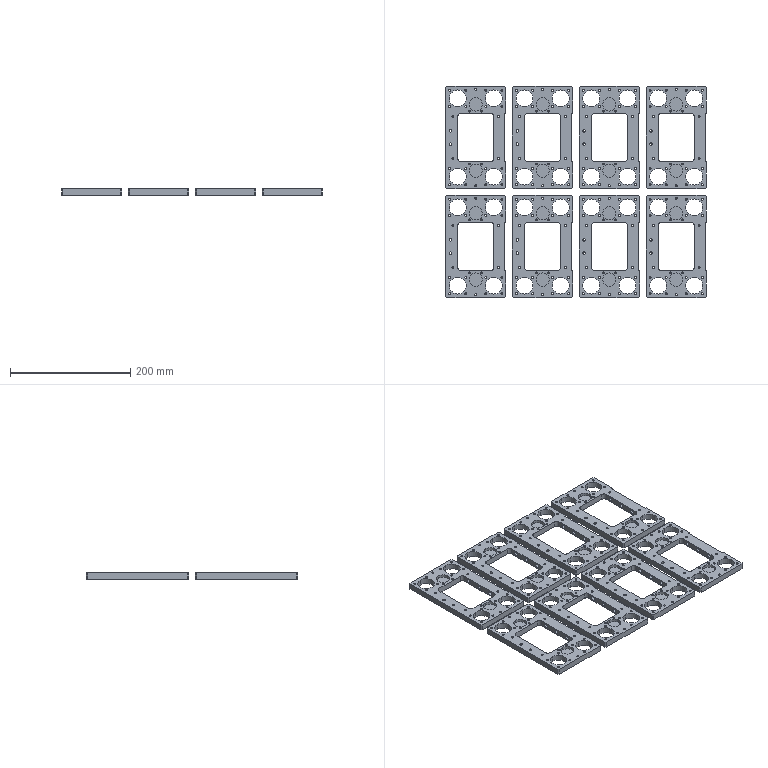NC program | NX | posted with a generic post | part box 433 x 351 x 10 mm
Lines 8361 to 9115 of 15742:
(ZLEVEL_PROFILE_COPY_COPY , TOOL : D10JING)
N16696 T14 M6
N16698 G54
N16700 G17 G0 G90 X191.064 Y-125.4 B0. C0. S9500 M3
N16702 G43 Z30. H14
N16704 Z-8.85
N16706 G94 G1 Z-9.85 F1000.
N16708 G3 X191.5 Y-125.5 R1.
N16710 G1 Y-55.5 F1500.
N16712 X141.623
N16714 X141.5
N16716 Y-125.5
N16718 X191.5
N16720 G3 X191.4 Y-125.064 R1.
N16722 G1 Z-8.85
N16724 G0 Z53.
N16726 X80.064 Y-125.4
N16728 Z-8.85
N16730 G1 Z-9.85 F1000.
N16732 G3 X80.5 Y-125.5 R1.
N16734 G1 Y-55.5 F1500.
N16736 X30.623
N16738 X30.5
N16740 Y-125.5
N16742 X80.5
N16744 G3 X80.4 Y-125.064 R1.
N16746 G1 Z-8.85
N16748 G0 Z53.
N16750 X-30.936 Y-125.4
N16752 Z-8.85
N16754 G1 Z-9.85 F1000.
N16756 G3 X-30.5 Y-125.5 R1.
N16758 G1 Y-55.5 F1500.
N16760 X-30.623
N16762 X-80.377
N16764 X-80.5
N16766 Y-125.5
N16768 X-30.5
N16770 G3 X-30.6 Y-125.064 R1.
N16772 G1 Z-8.85
N16774 G0 Z53.
N16776 X-191.065 Y-55.6
N16778 Z-8.85
N16780 G1 Z-9.85 F1000.
N16782 G3 X-191.5 Y-55.5 R1.
N16784 G1 Y-125.5 F1500.
N16786 X-141.5
N16788 Y-55.5
N16790 X-141.623
N16792 X-191.377
N16794 X-191.5
N16796 G3 X-191.4 Y-55.936 R1.
N16798 G1 Z-8.85
N16800 G0 Z53.
N16802 X-191.065 Y125.4
N16804 Z-8.85
N16806 G1 Z-9.85 F1000.
N16808 G3 X-191.5 Y125.5 R1.
N16810 G1 Y55.5 F1500.
N16812 X-141.5
N16814 Y125.5
N16816 X-141.623
N16818 X-191.377
N16820 X-191.5
N16822 G3 X-191.4 Y125.064 R1.
N16824 G1 Z-8.85
N16826 G0 Z53.
N16828 X-80.065 Y125.4
N16830 Z-8.85
N16832 G1 Z-9.85 F1000.
N16834 G3 X-80.5 Y125.5 R1.
N16836 G1 Y55.5 F1500.
N16838 X-30.5
N16840 Y125.5
N16842 X-30.623
N16844 X-80.377
N16846 X-80.5
N16848 G3 X-80.4 Y125.064 R1.
N16850 G1 Z-8.85
N16852 G0 Z53.
N16854 X30.935 Y125.4
N16856 Z-8.85
N16858 G1 Z-9.85 F1000.
N16860 G3 X30.5 Y125.5 R1.
N16862 G1 Y55.5 F1500.
N16864 X80.5
N16866 Y125.5
N16868 X80.377
N16870 X30.623
N16872 X30.5
N16874 G3 X30.6 Y125.064 R1.
N16876 G1 Z-8.85
N16878 G0 Z53.
N16880 X191.064 Y55.6
N16882 Z-8.85
N16884 G1 Z-9.85 F1000.
N16886 G3 X191.5 Y55.5 R1.
N16888 G1 Y125.5 F1500.
N16890 X191.377
N16892 X141.623
N16894 X141.5
N16896 Y55.5
N16898 X191.5
N16900 G3 X191.4 Y55.936 R1.
N16902 G1 Z-8.85
N16904 G0 Z30.
(HOLE_MILLING , TOOL : D10JING)
N16906 X-196.5 Y-155.5
N16908 Z0.5
N16910 G3 X-194.238 Y-157.763 R2.263 F2200.
N16912 X-191.975 Y-155.5 R2.263
N16914 X-191.975 Y-155.5 Z-0.38 I-4.525 J0.
N16916 X-191.975 Y-155.5 Z-1.26 I-4.525 J0.
N16918 X-191.975 Y-155.5 Z-2.14 I-4.525 J0.
N16920 X-191.975 Y-155.5 Z-3.02 I-4.525 J0.
N16922 X-191.975 Y-155.5 Z-3.9 I-4.525 J0.
N16924 X-191.975 Y-155.5 Z-4.78 I-4.525 J0.
N16926 X-191.975 Y-155.5 Z-5.66 I-4.525 J0.
N16928 X-191.975 Y-155.5 Z-6.54 I-4.525 J0.
N16930 X-191.975 Y-155.5 Z-7.42 I-4.525 J0.
N16932 X-191.975 Y-155.5 Z-8.3 I-4.525 J0.
N16934 X-191.975 Y-155.5 Z-9.18 I-4.525 J0.
N16936 X-192.384 Y-157.38 Z-10. R-4.525
N16938 X-194.62 Y-151.384 R4.525
N16940 X-192.384 Y-157.38 R-4.525
N16942 X-193.502 Y-154.382 R2.263
N16944 X-196.5 Y-155.5 R2.263
N16946 G0 Z0.5
N16948 G3 X-191.975 Y-160.025 R4.525
N16950 X-187.45 Y-155.5 R4.525
N16952 X-187.45 Y-155.5 Z-0.38 I-9.05 J0.
N16954 X-187.45 Y-155.5 Z-1.26 I-9.05 J0.
N16956 X-187.45 Y-155.5 Z-2.14 I-9.05 J0.
N16958 X-187.45 Y-155.5 Z-3.02 I-9.05 J0.
N16960 X-187.45 Y-155.5 Z-3.9 I-9.05 J0.
N16962 X-187.45 Y-155.5 Z-4.78 I-9.05 J0.
N16964 X-187.45 Y-155.5 Z-5.66 I-9.05 J0.
N16966 X-187.45 Y-155.5 Z-6.54 I-9.05 J0.
N16968 X-187.45 Y-155.5 Z-7.42 I-9.05 J0.
N16970 X-187.45 Y-155.5 Z-8.3 I-9.05 J0.
N16972 X-187.45 Y-155.5 Z-9.18 I-9.05 J0.
N16974 X-188.268 Y-159.26 Z-10. R-9.05
N16976 X-192.74 Y-147.268 R9.05
N16978 X-188.268 Y-159.26 R-9.05
N16980 X-190.504 Y-153.264 R4.525
N16982 X-196.5 Y-155.5 R4.525
N16984 G0 Z30.
N16986 X-166.5 Y-145.5
N16988 Z0.5
N16990 G3 X-165. Y-147. R1.5
N16992 X-163.5 Y-145.5 R1.5
N16994 X-163.5 Y-145.5 Z-0.38 I-3. J0.
N16996 X-163.5 Y-145.5 Z-1.26 I-3. J0.
N16998 X-163.5 Y-145.5 Z-2.14 I-3. J0.
N17000 X-163.5 Y-145.5 Z-3.02 I-3. J0.
N17002 X-163.5 Y-145.5 Z-3.9 I-3. J0.
N17004 X-163.5 Y-145.5 Z-4.78 I-3. J0.
N17006 X-166.5 Y-142.5 Z-5. R3.
N17008 X-169.5 Y-145.5 R3.
N17010 X-166.5 Y-142.5 R-3.
N17012 X-168. Y-144. R1.5
N17014 X-166.5 Y-145.5 R1.5
N17016 G0 Z0.5
N17018 G3 X-163.5 Y-148.5 R3.
N17020 X-160.5 Y-145.5 R3.
N17022 X-160.5 Y-145.5 Z-0.38 I-6. J0.
N17024 X-160.5 Y-145.5 Z-1.26 I-6. J0.
N17026 X-160.5 Y-145.5 Z-2.14 I-6. J0.
N17028 X-160.5 Y-145.5 Z-3.02 I-6. J0.
N17030 X-160.5 Y-145.5 Z-3.9 I-6. J0.
N17032 X-160.5 Y-145.5 Z-4.78 I-6. J0.
N17034 X-166.5 Y-139.5 Z-5. R6.
N17036 X-172.5 Y-145.5 R6.
N17038 X-166.5 Y-139.5 R-6.
N17040 X-169.5 Y-142.5 R3.
N17042 X-166.5 Y-145.5 R3.
N17044 G0 Z30.
N17046 X-136.5 Y-155.5
N17048 Z0.5
N17050 G3 X-134.238 Y-157.763 R2.262
N17052 X-131.975 Y-155.5 R2.262
N17054 X-131.975 Y-155.5 Z-0.38 I-4.525 J0.
N17056 X-131.975 Y-155.5 Z-1.26 I-4.525 J0.
N17058 X-131.975 Y-155.5 Z-2.14 I-4.525 J0.
N17060 X-131.975 Y-155.5 Z-3.02 I-4.525 J0.
N17062 X-131.975 Y-155.5 Z-3.9 I-4.525 J0.
N17064 X-131.975 Y-155.5 Z-4.78 I-4.525 J0.
N17066 X-131.975 Y-155.5 Z-5.66 I-4.525 J0.
N17068 X-131.975 Y-155.5 Z-6.54 I-4.525 J0.
N17070 X-131.975 Y-155.5 Z-7.42 I-4.525 J0.
N17072 X-131.975 Y-155.5 Z-8.3 I-4.525 J0.
N17074 X-131.975 Y-155.5 Z-9.18 I-4.525 J0.
N17076 X-132.384 Y-157.38 Z-10. R-4.525
N17078 X-134.62 Y-151.384 R4.525
N17080 X-132.384 Y-157.38 R-4.525
N17082 X-133.502 Y-154.382 R2.263
N17084 X-136.5 Y-155.5 R2.263
N17086 G0 Z0.5
N17088 G3 X-131.975 Y-160.025 R4.525
N17090 X-127.45 Y-155.5 R4.525
N17092 X-127.45 Y-155.5 Z-0.38 I-9.05 J0.
N17094 X-127.45 Y-155.5 Z-1.26 I-9.05 J0.
N17096 X-127.45 Y-155.5 Z-2.14 I-9.05 J0.
N17098 X-127.45 Y-155.5 Z-3.02 I-9.05 J0.
N17100 X-127.45 Y-155.5 Z-3.9 I-9.05 J0.
N17102 X-127.45 Y-155.5 Z-4.78 I-9.05 J0.
N17104 X-127.45 Y-155.5 Z-5.66 I-9.05 J0.
N17106 X-127.45 Y-155.5 Z-6.54 I-9.05 J0.
N17108 X-127.45 Y-155.5 Z-7.42 I-9.05 J0.
N17110 X-127.45 Y-155.5 Z-8.3 I-9.05 J0.
N17112 X-127.45 Y-155.5 Z-9.18 I-9.05 J0.
N17114 X-128.268 Y-159.26 Z-10. R-9.05
N17116 X-132.74 Y-147.268 R9.05
N17118 X-128.268 Y-159.26 R-9.05
N17120 X-130.504 Y-153.264 R4.525
N17122 X-136.5 Y-155.5 R4.525
N17124 G0 Z30.
N17126 X-85.5
N17128 Z0.5
N17130 G3 X-83.238 Y-157.763 R2.263
N17132 X-80.975 Y-155.5 R2.263
N17134 X-80.975 Y-155.5 Z-0.38 I-4.525 J0.
N17136 X-80.975 Y-155.5 Z-1.26 I-4.525 J0.
N17138 X-80.975 Y-155.5 Z-2.14 I-4.525 J0.
N17140 X-80.975 Y-155.5 Z-3.02 I-4.525 J0.
N17142 X-80.975 Y-155.5 Z-3.9 I-4.525 J0.
N17144 X-80.975 Y-155.5 Z-4.78 I-4.525 J0.
N17146 X-80.975 Y-155.5 Z-5.66 I-4.525 J0.
N17148 X-80.975 Y-155.5 Z-6.54 I-4.525 J0.
N17150 X-80.975 Y-155.5 Z-7.42 I-4.525 J0.
N17152 X-80.975 Y-155.5 Z-8.3 I-4.525 J0.
N17154 X-80.975 Y-155.5 Z-9.18 I-4.525 J0.
N17156 X-81.384 Y-157.38 Z-10. R-4.525
N17158 X-83.62 Y-151.384 R4.525
N17160 X-81.384 Y-157.38 R-4.525
N17162 X-82.502 Y-154.382 R2.263
N17164 X-85.5 Y-155.5 R2.263
N17166 G0 Z0.5
N17168 G3 X-80.975 Y-160.025 R4.525
N17170 X-76.45 Y-155.5 R4.525
N17172 X-76.45 Y-155.5 Z-0.38 I-9.05 J0.
N17174 X-76.45 Y-155.5 Z-1.26 I-9.05 J0.
N17176 X-76.45 Y-155.5 Z-2.14 I-9.05 J0.
N17178 X-76.45 Y-155.5 Z-3.02 I-9.05 J0.
N17180 X-76.45 Y-155.5 Z-3.9 I-9.05 J0.
N17182 X-76.45 Y-155.5 Z-4.78 I-9.05 J0.
N17184 X-76.45 Y-155.5 Z-5.66 I-9.05 J0.
N17186 X-76.45 Y-155.5 Z-6.54 I-9.05 J0.
N17188 X-76.45 Y-155.5 Z-7.42 I-9.05 J0.
N17190 X-76.45 Y-155.5 Z-8.3 I-9.05 J0.
N17192 X-76.45 Y-155.5 Z-9.18 I-9.05 J0.
N17194 X-77.268 Y-159.26 Z-10. R-9.05
N17196 X-81.74 Y-147.268 R9.05
N17198 X-77.268 Y-159.26 R-9.05
N17200 X-79.504 Y-153.264 R4.525
N17202 X-85.5 Y-155.5 R4.525
N17204 G0 Z30.
N17206 X-55.5 Y-145.5
N17208 Z0.5
N17210 G3 X-54. Y-147. R1.5
N17212 X-52.5 Y-145.5 R1.5
N17214 X-52.5 Y-145.5 Z-0.38 I-3. J0.
N17216 X-52.5 Y-145.5 Z-1.26 I-3. J0.
N17218 X-52.5 Y-145.5 Z-2.14 I-3. J0.
N17220 X-52.5 Y-145.5 Z-3.02 I-3. J0.
N17222 X-52.5 Y-145.5 Z-3.9 I-3. J0.
N17224 X-52.5 Y-145.5 Z-4.78 I-3. J0.
N17226 X-55.5 Y-142.5 Z-5. R3.
N17228 X-58.5 Y-145.5 R3.
N17230 X-55.5 Y-142.5 R-3.
N17232 X-57. Y-144. R1.5
N17234 X-55.5 Y-145.5 R1.5
N17236 G0 Z0.5
N17238 G3 X-52.5 Y-148.5 R3.
N17240 X-49.5 Y-145.5 R3.
N17242 X-49.5 Y-145.5 Z-0.38 I-6. J0.
N17244 X-49.5 Y-145.5 Z-1.26 I-6. J0.
N17246 X-49.5 Y-145.5 Z-2.14 I-6. J0.
N17248 X-49.5 Y-145.5 Z-3.02 I-6. J0.
N17250 X-49.5 Y-145.5 Z-3.9 I-6. J0.
N17252 X-49.5 Y-145.5 Z-4.78 I-6. J0.
N17254 X-55.5 Y-139.5 Z-5. R6.
N17256 X-61.5 Y-145.5 R6.
N17258 X-55.5 Y-139.5 R-6.
N17260 X-58.5 Y-142.5 R3.
N17262 X-55.5 Y-145.5 R3.
N17264 G0 Z30.
N17266 X-25.5 Y-155.5
N17268 Z0.5
N17270 G3 X-23.238 Y-157.763 R2.263
N17272 X-20.975 Y-155.5 R2.263
N17274 X-20.975 Y-155.5 Z-0.38 I-4.525 J0.
N17276 X-20.975 Y-155.5 Z-1.26 I-4.525 J0.
N17278 X-20.975 Y-155.5 Z-2.14 I-4.525 J0.
N17280 X-20.975 Y-155.5 Z-3.02 I-4.525 J0.
N17282 X-20.975 Y-155.5 Z-3.9 I-4.525 J0.
N17284 X-20.975 Y-155.5 Z-4.78 I-4.525 J0.
N17286 X-20.975 Y-155.5 Z-5.66 I-4.525 J0.
N17288 X-20.975 Y-155.5 Z-6.54 I-4.525 J0.
N17290 X-20.975 Y-155.5 Z-7.42 I-4.525 J0.
N17292 X-20.975 Y-155.5 Z-8.3 I-4.525 J0.
N17294 X-20.975 Y-155.5 Z-9.18 I-4.525 J0.
N17296 X-21.384 Y-157.38 Z-10. R-4.525
N17298 X-23.62 Y-151.384 R4.525
N17300 X-21.384 Y-157.38 R-4.525
N17302 X-22.502 Y-154.382 R2.263
N17304 X-25.5 Y-155.5 R2.263
N17306 G0 Z0.5
N17308 G3 X-20.975 Y-160.025 R4.525
N17310 X-16.45 Y-155.5 R4.525
N17312 X-16.45 Y-155.5 Z-0.38 I-9.05 J0.
N17314 X-16.45 Y-155.5 Z-1.26 I-9.05 J0.
N17316 X-16.45 Y-155.5 Z-2.14 I-9.05 J0.
N17318 X-16.45 Y-155.5 Z-3.02 I-9.05 J0.
N17320 X-16.45 Y-155.5 Z-3.9 I-9.05 J0.
N17322 X-16.45 Y-155.5 Z-4.78 I-9.05 J0.
N17324 X-16.45 Y-155.5 Z-5.66 I-9.05 J0.
N17326 X-16.45 Y-155.5 Z-6.54 I-9.05 J0.
N17328 X-16.45 Y-155.5 Z-7.42 I-9.05 J0.
N17330 X-16.45 Y-155.5 Z-8.3 I-9.05 J0.
N17332 X-16.45 Y-155.5 Z-9.18 I-9.05 J0.
N17334 X-17.268 Y-159.26 Z-10. R-9.05
N17336 X-21.74 Y-147.268 R9.05
N17338 X-17.268 Y-159.26 R-9.05
N17340 X-19.504 Y-153.264 R4.525
N17342 X-25.5 Y-155.5 R4.525
N17344 G0 Z30.
N17346 X25.5
N17348 Z0.5
N17350 G3 X27.763 Y-157.763 R2.263
N17352 X30.025 Y-155.5 R2.263
N17354 X30.025 Y-155.5 Z-0.38 I-4.525 J0.
N17356 X30.025 Y-155.5 Z-1.26 I-4.525 J0.
N17358 X30.025 Y-155.5 Z-2.14 I-4.525 J0.
N17360 X30.025 Y-155.5 Z-3.02 I-4.525 J0.
N17362 X30.025 Y-155.5 Z-3.9 I-4.525 J0.
N17364 X30.025 Y-155.5 Z-4.78 I-4.525 J0.
N17366 X30.025 Y-155.5 Z-5.66 I-4.525 J0.
N17368 X30.025 Y-155.5 Z-6.54 I-4.525 J0.
N17370 X30.025 Y-155.5 Z-7.42 I-4.525 J0.
N17372 X30.025 Y-155.5 Z-8.3 I-4.525 J0.
N17374 X30.025 Y-155.5 Z-9.18 I-4.525 J0.
N17376 X29.616 Y-157.38 Z-10. R-4.525
N17378 X27.38 Y-151.384 R4.525
N17380 X29.616 Y-157.38 R-4.525
N17382 X28.498 Y-154.382 R2.263
N17384 X25.5 Y-155.5 R2.263
N17386 G0 Z0.5
N17388 G3 X30.025 Y-160.025 R4.525
N17390 X34.55 Y-155.5 R4.525
N17392 X34.55 Y-155.5 Z-0.38 I-9.05 J0.
N17394 X34.55 Y-155.5 Z-1.26 I-9.05 J0.
N17396 X34.55 Y-155.5 Z-2.14 I-9.05 J0.
N17398 X34.55 Y-155.5 Z-3.02 I-9.05 J0.
N17400 X34.55 Y-155.5 Z-3.9 I-9.05 J0.
N17402 X34.55 Y-155.5 Z-4.78 I-9.05 J0.
N17404 X34.55 Y-155.5 Z-5.66 I-9.05 J0.
N17406 X34.55 Y-155.5 Z-6.54 I-9.05 J0.
N17408 X34.55 Y-155.5 Z-7.42 I-9.05 J0.
N17410 X34.55 Y-155.5 Z-8.3 I-9.05 J0.
N17412 X34.55 Y-155.5 Z-9.18 I-9.05 J0.
N17414 X33.732 Y-159.26 Z-10. R-9.05
N17416 X29.26 Y-147.268 R9.05
N17418 X33.732 Y-159.26 R-9.05
N17420 X31.496 Y-153.264 R4.525
N17422 X25.5 Y-155.5 R4.525
N17424 G0 Z30.
N17426 X55.5 Y-145.5
N17428 Z0.5
N17430 G3 X57. Y-147. R1.5
N17432 X58.5 Y-145.5 R1.5
N17434 X58.5 Y-145.5 Z-0.38 I-3. J0.
N17436 X58.5 Y-145.5 Z-1.26 I-3. J0.
N17438 X58.5 Y-145.5 Z-2.14 I-3. J0.
N17440 X58.5 Y-145.5 Z-3.02 I-3. J0.
N17442 X58.5 Y-145.5 Z-3.9 I-3. J0.
N17444 X58.5 Y-145.5 Z-4.78 I-3. J0.
N17446 X55.5 Y-142.5 Z-5. R3.
N17448 X52.5 Y-145.5 R3.
N17450 X55.5 Y-142.5 R-3.
N17452 X54. Y-144. R1.5
N17454 X55.5 Y-145.5 R1.5
N17456 G0 Z0.5
N17458 G3 X58.5 Y-148.5 R3.
N17460 X61.5 Y-145.5 R3.
N17462 X61.5 Y-145.5 Z-0.38 I-6. J0.
N17464 X61.5 Y-145.5 Z-1.26 I-6. J0.
N17466 X61.5 Y-145.5 Z-2.14 I-6. J0.
N17468 X61.5 Y-145.5 Z-3.02 I-6. J0.
N17470 X61.5 Y-145.5 Z-3.9 I-6. J0.
N17472 X61.5 Y-145.5 Z-4.78 I-6. J0.
N17474 X55.5 Y-139.5 Z-5. R6.
N17476 X49.5 Y-145.5 R6.
N17478 X55.5 Y-139.5 R-6.
N17480 X52.5 Y-142.5 R3.
N17482 X55.5 Y-145.5 R3.
N17484 G0 Z30.
N17486 X85.5 Y-155.5
N17488 Z0.5
N17490 G3 X87.763 Y-157.763 R2.262
N17492 X90.025 Y-155.5 R2.262
N17494 X90.025 Y-155.5 Z-0.38 I-4.525 J0.
N17496 X90.025 Y-155.5 Z-1.26 I-4.525 J0.
N17498 X90.025 Y-155.5 Z-2.14 I-4.525 J0.
N17500 X90.025 Y-155.5 Z-3.02 I-4.525 J0.
N17502 X90.025 Y-155.5 Z-3.9 I-4.525 J0.
N17504 X90.025 Y-155.5 Z-4.78 I-4.525 J0.
N17506 X90.025 Y-155.5 Z-5.66 I-4.525 J0.
N17508 X90.025 Y-155.5 Z-6.54 I-4.525 J0.
N17510 X90.025 Y-155.5 Z-7.42 I-4.525 J0.
N17512 X90.025 Y-155.5 Z-8.3 I-4.525 J0.
N17514 X90.025 Y-155.5 Z-9.18 I-4.525 J0.
N17516 X89.616 Y-157.38 Z-10. R-4.525
N17518 X87.38 Y-151.384 R4.525
N17520 X89.616 Y-157.38 R-4.525
N17522 X88.498 Y-154.382 R2.263
N17524 X85.5 Y-155.5 R2.263
N17526 G0 Z0.5
N17528 G3 X90.025 Y-160.025 R4.525
N17530 X94.55 Y-155.5 R4.525
N17532 X94.55 Y-155.5 Z-0.38 I-9.05 J0.
N17534 X94.55 Y-155.5 Z-1.26 I-9.05 J0.
N17536 X94.55 Y-155.5 Z-2.14 I-9.05 J0.
N17538 X94.55 Y-155.5 Z-3.02 I-9.05 J0.
N17540 X94.55 Y-155.5 Z-3.9 I-9.05 J0.
N17542 X94.55 Y-155.5 Z-4.78 I-9.05 J0.
N17544 X94.55 Y-155.5 Z-5.66 I-9.05 J0.
N17546 X94.55 Y-155.5 Z-6.54 I-9.05 J0.
N17548 X94.55 Y-155.5 Z-7.42 I-9.05 J0.
N17550 X94.55 Y-155.5 Z-8.3 I-9.05 J0.
N17552 X94.55 Y-155.5 Z-9.18 I-9.05 J0.
N17554 X93.732 Y-159.26 Z-10. R-9.05
N17556 X89.26 Y-147.268 R9.05
N17558 X93.732 Y-159.26 R-9.05
N17560 X91.496 Y-153.264 R4.525
N17562 X85.5 Y-155.5 R4.525
N17564 G0 Z30.
N17566 X136.5
N17568 Z0.5
N17570 G3 X138.763 Y-157.763 R2.262
N17572 X141.025 Y-155.5 R2.262
N17574 X141.025 Y-155.5 Z-0.38 I-4.525 J0.
N17576 X141.025 Y-155.5 Z-1.26 I-4.525 J0.
N17578 X141.025 Y-155.5 Z-2.14 I-4.525 J0.
N17580 X141.025 Y-155.5 Z-3.02 I-4.525 J0.
N17582 X141.025 Y-155.5 Z-3.9 I-4.525 J0.
N17584 X141.025 Y-155.5 Z-4.78 I-4.525 J0.
N17586 X141.025 Y-155.5 Z-5.66 I-4.525 J0.
N17588 X141.025 Y-155.5 Z-6.54 I-4.525 J0.
N17590 X141.025 Y-155.5 Z-7.42 I-4.525 J0.
N17592 X141.025 Y-155.5 Z-8.3 I-4.525 J0.
N17594 X141.025 Y-155.5 Z-9.18 I-4.525 J0.
N17596 X140.616 Y-157.38 Z-10. R-4.525
N17598 X138.38 Y-151.384 R4.525
N17600 X140.616 Y-157.38 R-4.525
N17602 X139.498 Y-154.382 R2.263
N17604 X136.5 Y-155.5 R2.263
N17606 G0 Z0.5
N17608 G3 X141.025 Y-160.025 R4.525
N17610 X145.55 Y-155.5 R4.525
N17612 X145.55 Y-155.5 Z-0.38 I-9.05 J0.
N17614 X145.55 Y-155.5 Z-1.26 I-9.05 J0.
N17616 X145.55 Y-155.5 Z-2.14 I-9.05 J0.
N17618 X145.55 Y-155.5 Z-3.02 I-9.05 J0.
N17620 X145.55 Y-155.5 Z-3.9 I-9.05 J0.
N17622 X145.55 Y-155.5 Z-4.78 I-9.05 J0.
N17624 X145.55 Y-155.5 Z-5.66 I-9.05 J0.
N17626 X145.55 Y-155.5 Z-6.54 I-9.05 J0.
N17628 X145.55 Y-155.5 Z-7.42 I-9.05 J0.
N17630 X145.55 Y-155.5 Z-8.3 I-9.05 J0.
N17632 X145.55 Y-155.5 Z-9.18 I-9.05 J0.
N17634 X144.732 Y-159.26 Z-10. R-9.05
N17636 X140.26 Y-147.268 R9.05
N17638 X144.732 Y-159.26 R-9.05
N17640 X142.496 Y-153.264 R4.525
N17642 X136.5 Y-155.5 R4.525
N17644 G0 Z30.
N17646 X166.5 Y-145.5
N17648 Z0.5
N17650 G3 X168. Y-147. R1.5
N17652 X169.5 Y-145.5 R1.5
N17654 X169.5 Y-145.5 Z-0.38 I-3. J0.
N17656 X169.5 Y-145.5 Z-1.26 I-3. J0.
N17658 X169.5 Y-145.5 Z-2.14 I-3. J0.
N17660 X169.5 Y-145.5 Z-3.02 I-3. J0.
N17662 X169.5 Y-145.5 Z-3.9 I-3. J0.
N17664 X169.5 Y-145.5 Z-4.78 I-3. J0.
N17666 X166.5 Y-142.5 Z-5. R3.
N17668 X163.5 Y-145.5 R3.
N17670 X166.5 Y-142.5 R-3.
N17672 X165. Y-144. R1.5
N17674 X166.5 Y-145.5 R1.5
N17676 G0 Z0.5
N17678 G3 X169.5 Y-148.5 R3.
N17680 X172.5 Y-145.5 R3.
N17682 X172.5 Y-145.5 Z-0.38 I-6. J0.
N17684 X172.5 Y-145.5 Z-1.26 I-6. J0.
N17686 X172.5 Y-145.5 Z-2.14 I-6. J0.
N17688 X172.5 Y-145.5 Z-3.02 I-6. J0.
N17690 X172.5 Y-145.5 Z-3.9 I-6. J0.
N17692 X172.5 Y-145.5 Z-4.78 I-6. J0.
N17694 X166.5 Y-139.5 Z-5. R6.
N17696 X160.5 Y-145.5 R6.
N17698 X166.5 Y-139.5 R-6.
N17700 X163.5 Y-142.5 R3.
N17702 X166.5 Y-145.5 R3.
N17704 G0 Z30.
N17706 X196.5 Y-155.5
N17708 Z0.5
N17710 G3 X198.763 Y-157.763 R2.262
N17712 X201.025 Y-155.5 R2.262
N17714 X201.025 Y-155.5 Z-0.38 I-4.525 J0.
N17716 X201.025 Y-155.5 Z-1.26 I-4.525 J0.
N17718 X201.025 Y-155.5 Z-2.14 I-4.525 J0.
N17720 X201.025 Y-155.5 Z-3.02 I-4.525 J0.
N17722 X201.025 Y-155.5 Z-3.9 I-4.525 J0.
N17724 X201.025 Y-155.5 Z-4.78 I-4.525 J0.
N17726 X201.025 Y-155.5 Z-5.66 I-4.525 J0.
N17728 X201.025 Y-155.5 Z-6.54 I-4.525 J0.
N17730 X201.025 Y-155.5 Z-7.42 I-4.525 J0.
N17732 X201.025 Y-155.5 Z-8.3 I-4.525 J0.
N17734 X201.025 Y-155.5 Z-9.18 I-4.525 J0.
N17736 X200.616 Y-157.38 Z-10. R-4.525
N17738 X198.38 Y-151.384 R4.525
N17740 X200.616 Y-157.38 R-4.525
N17742 X199.498 Y-154.382 R2.263
N17744 X196.5 Y-155.5 R2.263
N17746 G0 Z0.5
N17748 G3 X201.025 Y-160.025 R4.525
N17750 X205.55 Y-155.5 R4.525
N17752 X205.55 Y-155.5 Z-0.38 I-9.05 J0.
N17754 X205.55 Y-155.5 Z-1.26 I-9.05 J0.
N17756 X205.55 Y-155.5 Z-2.14 I-9.05 J0.
N17758 X205.55 Y-155.5 Z-3.02 I-9.05 J0.
N17760 X205.55 Y-155.5 Z-3.9 I-9.05 J0.
N17762 X205.55 Y-155.5 Z-4.78 I-9.05 J0.
N17764 X205.55 Y-155.5 Z-5.66 I-9.05 J0.
N17766 X205.55 Y-155.5 Z-6.54 I-9.05 J0.
N17768 X205.55 Y-155.5 Z-7.42 I-9.05 J0.
N17770 X205.55 Y-155.5 Z-8.3 I-9.05 J0.
N17772 X205.55 Y-155.5 Z-9.18 I-9.05 J0.
N17774 X204.732 Y-159.26 Z-10. R-9.05
N17776 X200.26 Y-147.268 R9.05
N17778 X204.732 Y-159.26 R-9.05
N17780 X202.496 Y-153.264 R4.525
N17782 X196.5 Y-155.5 R4.525
N17784 G0 Z30.
N17786 Y-25.5
N17788 Z0.5
N17790 G3 X198.763 Y-27.763 R2.262
N17792 X201.025 Y-25.5 R2.262
N17794 X201.025 Y-25.5 Z-0.38 I-4.525 J0.
N17796 X201.025 Y-25.5 Z-1.26 I-4.525 J0.
N17798 X201.025 Y-25.5 Z-2.14 I-4.525 J0.
N17800 X201.025 Y-25.5 Z-3.02 I-4.525 J0.
N17802 X201.025 Y-25.5 Z-3.9 I-4.525 J0.
N17804 X201.025 Y-25.5 Z-4.78 I-4.525 J0.
N17806 X201.025 Y-25.5 Z-5.66 I-4.525 J0.
N17808 X201.025 Y-25.5 Z-6.54 I-4.525 J0.
N17810 X201.025 Y-25.5 Z-7.42 I-4.525 J0.
N17812 X201.025 Y-25.5 Z-8.3 I-4.525 J0.
N17814 X201.025 Y-25.5 Z-9.18 I-4.525 J0.
N17816 X200.616 Y-27.38 Z-10. R-4.525
N17818 X198.38 Y-21.384 R4.525
N17820 X200.616 Y-27.38 R-4.525
N17822 X199.498 Y-24.382 R2.263
N17824 X196.5 Y-25.5 R2.263
N17826 G0 Z0.5
N17828 G3 X201.025 Y-30.025 R4.525
N17830 X205.55 Y-25.5 R4.525
N17832 X205.55 Y-25.5 Z-0.38 I-9.05 J0.
N17834 X205.55 Y-25.5 Z-1.26 I-9.05 J0.
N17836 X205.55 Y-25.5 Z-2.14 I-9.05 J0.
N17838 X205.55 Y-25.5 Z-3.02 I-9.05 J0.
N17840 X205.55 Y-25.5 Z-3.9 I-9.05 J0.
N17842 X205.55 Y-25.5 Z-4.78 I-9.05 J0.
N17844 X205.55 Y-25.5 Z-5.66 I-9.05 J0.
N17846 X205.55 Y-25.5 Z-6.54 I-9.05 J0.
N17848 X205.55 Y-25.5 Z-7.42 I-9.05 J0.
N17850 X205.55 Y-25.5 Z-8.3 I-9.05 J0.
N17852 X205.55 Y-25.5 Z-9.18 I-9.05 J0.
N17854 X204.732 Y-29.26 Z-10. R-9.05
N17856 X200.26 Y-17.268 R9.05
N17858 X204.732 Y-29.26 R-9.05
N17860 X202.496 Y-23.264 R4.525
N17862 X196.5 Y-25.5 R4.525
N17864 G0 Z30.
N17866 Y25.5
N17868 Z0.5
N17870 G3 X198.763 Y23.238 R2.262
N17872 X201.025 Y25.5 R2.262
N17874 X201.025 Y25.5 Z-0.38 I-4.525 J0.
N17876 X201.025 Y25.5 Z-1.26 I-4.525 J0.
N17878 X201.025 Y25.5 Z-2.14 I-4.525 J0.
N17880 X201.025 Y25.5 Z-3.02 I-4.525 J0.
N17882 X201.025 Y25.5 Z-3.9 I-4.525 J0.
N17884 X201.025 Y25.5 Z-4.78 I-4.525 J0.
N17886 X201.025 Y25.5 Z-5.66 I-4.525 J0.
N17888 X201.025 Y25.5 Z-6.54 I-4.525 J0.
N17890 X201.025 Y25.5 Z-7.42 I-4.525 J0.
N17892 X201.025 Y25.5 Z-8.3 I-4.525 J0.
N17894 X201.025 Y25.5 Z-9.18 I-4.525 J0.
N17896 X200.616 Y23.62 Z-10. R-4.525
N17898 X198.38 Y29.616 R4.525
N17900 X200.616 Y23.62 R-4.525
N17902 X199.498 Y26.618 R2.263
N17904 X196.5 Y25.5 R2.263
N17906 G0 Z0.5
N17908 G3 X201.025 Y20.975 R4.525
N17910 X205.55 Y25.5 R4.525
N17912 X205.55 Y25.5 Z-0.38 I-9.05 J0.
N17914 X205.55 Y25.5 Z-1.26 I-9.05 J0.
N17916 X205.55 Y25.5 Z-2.14 I-9.05 J0.
N17918 X205.55 Y25.5 Z-3.02 I-9.05 J0.
N17920 X205.55 Y25.5 Z-3.9 I-9.05 J0.
N17922 X205.55 Y25.5 Z-4.78 I-9.05 J0.
N17924 X205.55 Y25.5 Z-5.66 I-9.05 J0.
N17926 X205.55 Y25.5 Z-6.54 I-9.05 J0.
N17928 X205.55 Y25.5 Z-7.42 I-9.05 J0.
N17930 X205.55 Y25.5 Z-8.3 I-9.05 J0.
N17932 X205.55 Y25.5 Z-9.18 I-9.05 J0.
N17934 X204.732 Y21.74 Z-10. R-9.05
N17936 X200.26 Y33.732 R9.05
N17938 X204.732 Y21.74 R-9.05
N17940 X202.496 Y27.736 R4.525
N17942 X196.5 Y25.5 R4.525
N17944 G0 Z30.
N17946 X166.5 Y35.5
N17948 Z0.5
N17950 G3 X168. Y34. R1.5
N17952 X169.5 Y35.5 R1.5
N17954 X169.5 Y35.5 Z-0.38 I-3. J0.
N17956 X169.5 Y35.5 Z-1.26 I-3. J0.
N17958 X169.5 Y35.5 Z-2.14 I-3. J0.
N17960 X169.5 Y35.5 Z-3.02 I-3. J0.
N17962 X169.5 Y35.5 Z-3.9 I-3. J0.
N17964 X169.5 Y35.5 Z-4.78 I-3. J0.
N17966 X166.5 Y38.5 Z-5. R3.
N17968 X163.5 Y35.5 R3.
N17970 X166.5 Y38.5 R-3.
N17972 X165. Y37. R1.5
N17974 X166.5 Y35.5 R1.5
N17976 G0 Z0.5
N17978 G3 X169.5 Y32.5 R3.
N17980 X172.5 Y35.5 R3.
N17982 X172.5 Y35.5 Z-0.38 I-6. J0.
N17984 X172.5 Y35.5 Z-1.26 I-6. J0.
N17986 X172.5 Y35.5 Z-2.14 I-6. J0.
N17988 X172.5 Y35.5 Z-3.02 I-6. J0.
N17990 X172.5 Y35.5 Z-3.9 I-6. J0.
N17992 X172.5 Y35.5 Z-4.78 I-6. J0.
N17994 X166.5 Y41.5 Z-5. R6.
N17996 X160.5 Y35.5 R6.
N17998 X166.5 Y41.5 R-6.
N18000 X163.5 Y38.5 R3.
N18002 X166.5 Y35.5 R3.
N18004 G0 Z30.
N18006 X136.5 Y25.5
N18008 Z0.5
N18010 G3 X138.763 Y23.238 R2.262
N18012 X141.025 Y25.5 R2.262
N18014 X141.025 Y25.5 Z-0.38 I-4.525 J0.
N18016 X141.025 Y25.5 Z-1.26 I-4.525 J0.
N18018 X141.025 Y25.5 Z-2.14 I-4.525 J0.
N18020 X141.025 Y25.5 Z-3.02 I-4.525 J0.
N18022 X141.025 Y25.5 Z-3.9 I-4.525 J0.
N18024 X141.025 Y25.5 Z-4.78 I-4.525 J0.
N18026 X141.025 Y25.5 Z-5.66 I-4.525 J0.
N18028 X141.025 Y25.5 Z-6.54 I-4.525 J0.
N18030 X141.025 Y25.5 Z-7.42 I-4.525 J0.
N18032 X141.025 Y25.5 Z-8.3 I-4.525 J0.
N18034 X141.025 Y25.5 Z-9.18 I-4.525 J0.
N18036 X140.616 Y23.62 Z-10. R-4.525
N18038 X138.38 Y29.616 R4.525
N18040 X140.616 Y23.62 R-4.525
N18042 X139.498 Y26.618 R2.263
N18044 X136.5 Y25.5 R2.263
N18046 G0 Z0.5
N18048 G3 X141.025 Y20.975 R4.525
N18050 X145.55 Y25.5 R4.525
N18052 X145.55 Y25.5 Z-0.38 I-9.05 J0.
N18054 X145.55 Y25.5 Z-1.26 I-9.05 J0.
N18056 X145.55 Y25.5 Z-2.14 I-9.05 J0.
N18058 X145.55 Y25.5 Z-3.02 I-9.05 J0.
N18060 X145.55 Y25.5 Z-3.9 I-9.05 J0.
N18062 X145.55 Y25.5 Z-4.78 I-9.05 J0.
N18064 X145.55 Y25.5 Z-5.66 I-9.05 J0.
N18066 X145.55 Y25.5 Z-6.54 I-9.05 J0.
N18068 X145.55 Y25.5 Z-7.42 I-9.05 J0.
N18070 X145.55 Y25.5 Z-8.3 I-9.05 J0.
N18072 X145.55 Y25.5 Z-9.18 I-9.05 J0.
N18074 X144.732 Y21.74 Z-10. R-9.05
N18076 X140.26 Y33.732 R9.05
N18078 X144.732 Y21.74 R-9.05
N18080 X142.496 Y27.736 R4.525
N18082 X136.5 Y25.5 R4.525
N18084 G0 Z30.
N18086 X166.5 Y-35.5
N18088 Z0.5
N18090 G3 X168. Y-37. R1.5
N18092 X169.5 Y-35.5 R1.5
N18094 X169.5 Y-35.5 Z-0.38 I-3. J0.
N18096 X169.5 Y-35.5 Z-1.26 I-3. J0.
N18098 X169.5 Y-35.5 Z-2.14 I-3. J0.
N18100 X169.5 Y-35.5 Z-3.02 I-3. J0.
N18102 X169.5 Y-35.5 Z-3.9 I-3. J0.
N18104 X169.5 Y-35.5 Z-4.78 I-3. J0.
N18106 X166.5 Y-32.5 Z-5. R3.
N18108 X163.5 Y-35.5 R3.
N18110 X166.5 Y-32.5 R-3.
N18112 X165. Y-34. R1.5
N18114 X166.5 Y-35.5 R1.5
N18116 G0 Z0.5
N18118 G3 X169.5 Y-38.5 R3.
N18120 X172.5 Y-35.5 R3.
N18122 X172.5 Y-35.5 Z-0.38 I-6. J0.
N18124 X172.5 Y-35.5 Z-1.26 I-6. J0.
N18126 X172.5 Y-35.5 Z-2.14 I-6. J0.
N18128 X172.5 Y-35.5 Z-3.02 I-6. J0.
N18130 X172.5 Y-35.5 Z-3.9 I-6. J0.
N18132 X172.5 Y-35.5 Z-4.78 I-6. J0.
N18134 X166.5 Y-29.5 Z-5. R6.
N18136 X160.5 Y-35.5 R6.
N18138 X166.5 Y-29.5 R-6.
N18140 X163.5 Y-32.5 R3.
N18142 X166.5 Y-35.5 R3.
N18144 G0 Z30.
N18146 X136.5 Y-25.5
N18148 Z0.5
N18150 G3 X138.763 Y-27.763 R2.262
N18152 X141.025 Y-25.5 R2.262
N18154 X141.025 Y-25.5 Z-0.38 I-4.525 J0.
N18156 X141.025 Y-25.5 Z-1.26 I-4.525 J0.
N18158 X141.025 Y-25.5 Z-2.14 I-4.525 J0.
N18160 X141.025 Y-25.5 Z-3.02 I-4.525 J0.
N18162 X141.025 Y-25.5 Z-3.9 I-4.525 J0.
N18164 X141.025 Y-25.5 Z-4.78 I-4.525 J0.
N18166 X141.025 Y-25.5 Z-5.66 I-4.525 J0.
N18168 X141.025 Y-25.5 Z-6.54 I-4.525 J0.
N18170 X141.025 Y-25.5 Z-7.42 I-4.525 J0.
N18172 X141.025 Y-25.5 Z-8.3 I-4.525 J0.
N18174 X141.025 Y-25.5 Z-9.18 I-4.525 J0.
N18176 X140.616 Y-27.38 Z-10. R-4.525
N18178 X138.38 Y-21.384 R4.525
N18180 X140.616 Y-27.38 R-4.525
N18182 X139.498 Y-24.382 R2.263
N18184 X136.5 Y-25.5 R2.263
N18186 G0 Z0.5
N18188 G3 X141.025 Y-30.025 R4.525
N18190 X145.55 Y-25.5 R4.525
N18192 X145.55 Y-25.5 Z-0.38 I-9.05 J0.